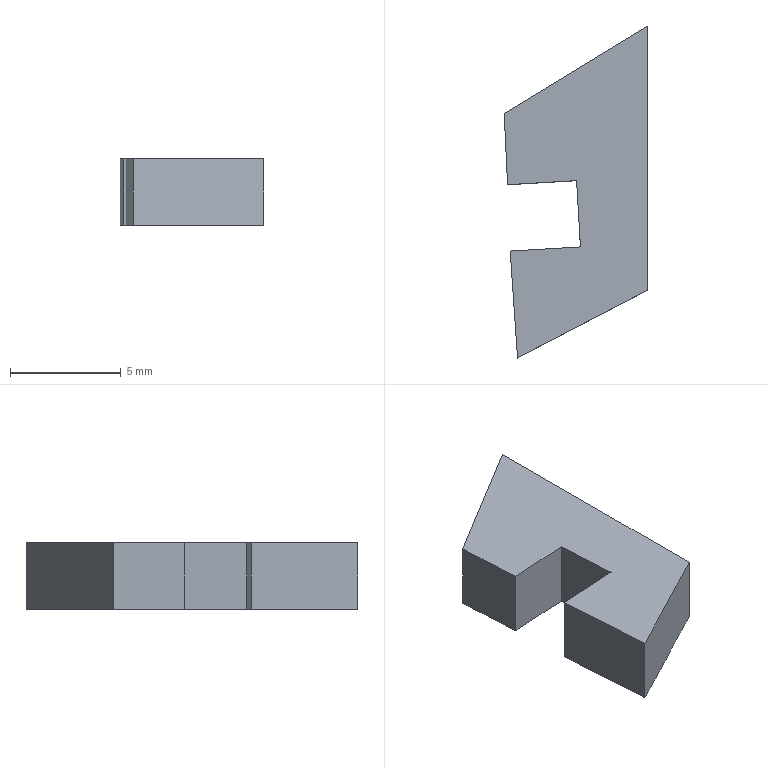Part | SolidWorks | features BaseBody 1 | 1 solid | 10 faces | box 6.477 x 14.965 x 3 mm | volume 188.364 mm3 | plane 10
STEP:
#1=CARTESIAN_POINT('',(10.676,5.598,-1.5));
#2=VERTEX_POINT('',#1);
#3=CARTESIAN_POINT('',(7.509,5.413,-1.5));
#4=VERTEX_POINT('',#3);
#5=CARTESIAN_POINT('',(7.509,5.413,-1.5));
#6=DIRECTION('',(-0.9983,-0.05835,0.));
#7=VECTOR('',#6,1000.);
#8=LINE('',#5,#7);
#9=EDGE_CURVE('',#2,#4,#8,.T.);
#10=ORIENTED_EDGE('',*,*,#9,.F.);
#11=CARTESIAN_POINT('',(10.501,8.588,-1.5));
#12=VERTEX_POINT('',#11);
#13=CARTESIAN_POINT('',(10.676,5.598,-1.5));
#14=DIRECTION('',(0.05835,-0.9983,0.));
#15=VECTOR('',#14,1000.);
#16=LINE('',#13,#15);
#17=EDGE_CURVE('',#12,#2,#16,.T.);
#18=ORIENTED_EDGE('',*,*,#17,.F.);
#19=CARTESIAN_POINT('',(7.389,8.407,-1.5));
#20=VERTEX_POINT('',#19);
#21=CARTESIAN_POINT('',(10.501,8.588,-1.5));
#22=DIRECTION('',(0.9983,0.05835,0.));
#23=VECTOR('',#22,1000.);
#24=LINE('',#21,#23);
#25=EDGE_CURVE('',#20,#12,#24,.T.);
#26=ORIENTED_EDGE('',*,*,#25,.F.);
#27=CARTESIAN_POINT('',(7.239,11.616,-1.5));
#28=VERTEX_POINT('',#27);
#29=CARTESIAN_POINT('',(7.389,8.407,-1.5));
#30=DIRECTION('',(0.04694,-0.9989,0.));
#31=VECTOR('',#30,1000.);
#32=LINE('',#29,#31);
#33=EDGE_CURVE('',#28,#20,#32,.T.);
#34=ORIENTED_EDGE('',*,*,#33,.F.);
#35=CARTESIAN_POINT('',(13.715,15.561,-1.5));
#36=VERTEX_POINT('',#35);
#37=CARTESIAN_POINT('',(7.239,11.616,-1.5));
#38=DIRECTION('',(-0.854,-0.5202,0.));
#39=VECTOR('',#38,1000.);
#40=LINE('',#37,#39);
#41=EDGE_CURVE('',#36,#28,#40,.T.);
#42=ORIENTED_EDGE('',*,*,#41,.F.);
#43=CARTESIAN_POINT('',(13.715,3.649,-1.5));
#44=VERTEX_POINT('',#43);
#45=CARTESIAN_POINT('',(13.715,15.561,-1.5));
#46=DIRECTION('',(0.,1.,0.));
#47=VECTOR('',#46,1000.);
#48=LINE('',#45,#47);
#49=EDGE_CURVE('',#44,#36,#48,.T.);
#50=ORIENTED_EDGE('',*,*,#49,.F.);
#51=CARTESIAN_POINT('',(7.839,0.5953,-1.5));
#52=VERTEX_POINT('',#51);
#53=CARTESIAN_POINT('',(13.715,3.649,-1.5));
#54=DIRECTION('',(0.8874,0.4611,0.));
#55=VECTOR('',#54,1000.);
#56=LINE('',#53,#55);
#57=EDGE_CURVE('',#52,#44,#56,.T.);
#58=ORIENTED_EDGE('',*,*,#57,.F.);
#59=CARTESIAN_POINT('',(7.839,0.5953,-1.5));
#60=DIRECTION('',(0.06826,-0.9977,0.));
#61=VECTOR('',#60,1000.);
#62=LINE('',#59,#61);
#63=EDGE_CURVE('',#4,#52,#62,.T.);
#64=ORIENTED_EDGE('',*,*,#63,.F.);
#65=EDGE_LOOP('',(#10,#18,#26,#34,#42,#50,#58,#64));
#66=FACE_OUTER_BOUND('',#65,.T.);
#67=CARTESIAN_POINT('',(0.,0.,-1.5));
#68=DIRECTION('',(0.,0.,1.));
#69=DIRECTION('',(1.,0.,0.));
#70=AXIS2_PLACEMENT_3D('',#67,#68,#69);
#71=PLANE('',#70);
#72=ADVANCED_FACE('',(#66),#71,.F.);
#73=CARTESIAN_POINT('',(10.676,5.598,1.5));
#74=VERTEX_POINT('',#73);
#75=CARTESIAN_POINT('',(7.509,5.413,1.5));
#76=VERTEX_POINT('',#75);
#77=CARTESIAN_POINT('',(7.509,5.413,1.5));
#78=DIRECTION('',(-0.9983,-0.05835,0.));
#79=VECTOR('',#78,1000.);
#80=LINE('',#77,#79);
#81=EDGE_CURVE('',#74,#76,#80,.T.);
#82=ORIENTED_EDGE('',*,*,#81,.T.);
#83=CARTESIAN_POINT('',(7.839,0.5953,1.5));
#84=VERTEX_POINT('',#83);
#85=CARTESIAN_POINT('',(7.839,0.5953,1.5));
#86=DIRECTION('',(0.06826,-0.9977,0.));
#87=VECTOR('',#86,1000.);
#88=LINE('',#85,#87);
#89=EDGE_CURVE('',#76,#84,#88,.T.);
#90=ORIENTED_EDGE('',*,*,#89,.T.);
#91=CARTESIAN_POINT('',(13.715,3.649,1.5));
#92=VERTEX_POINT('',#91);
#93=CARTESIAN_POINT('',(13.715,3.649,1.5));
#94=DIRECTION('',(0.8874,0.4611,0.));
#95=VECTOR('',#94,1000.);
#96=LINE('',#93,#95);
#97=EDGE_CURVE('',#84,#92,#96,.T.);
#98=ORIENTED_EDGE('',*,*,#97,.T.);
#99=CARTESIAN_POINT('',(13.715,15.561,1.5));
#100=VERTEX_POINT('',#99);
#101=CARTESIAN_POINT('',(13.715,15.561,1.5));
#102=DIRECTION('',(0.,1.,0.));
#103=VECTOR('',#102,1000.);
#104=LINE('',#101,#103);
#105=EDGE_CURVE('',#92,#100,#104,.T.);
#106=ORIENTED_EDGE('',*,*,#105,.T.);
#107=CARTESIAN_POINT('',(7.239,11.616,1.5));
#108=VERTEX_POINT('',#107);
#109=CARTESIAN_POINT('',(7.239,11.616,1.5));
#110=DIRECTION('',(-0.854,-0.5202,0.));
#111=VECTOR('',#110,1000.);
#112=LINE('',#109,#111);
#113=EDGE_CURVE('',#100,#108,#112,.T.);
#114=ORIENTED_EDGE('',*,*,#113,.T.);
#115=CARTESIAN_POINT('',(7.389,8.407,1.5));
#116=VERTEX_POINT('',#115);
#117=CARTESIAN_POINT('',(7.389,8.407,1.5));
#118=DIRECTION('',(0.04694,-0.9989,0.));
#119=VECTOR('',#118,1000.);
#120=LINE('',#117,#119);
#121=EDGE_CURVE('',#108,#116,#120,.T.);
#122=ORIENTED_EDGE('',*,*,#121,.T.);
#123=CARTESIAN_POINT('',(10.501,8.588,1.5));
#124=VERTEX_POINT('',#123);
#125=CARTESIAN_POINT('',(10.501,8.588,1.5));
#126=DIRECTION('',(0.9983,0.05835,0.));
#127=VECTOR('',#126,1000.);
#128=LINE('',#125,#127);
#129=EDGE_CURVE('',#116,#124,#128,.T.);
#130=ORIENTED_EDGE('',*,*,#129,.T.);
#131=CARTESIAN_POINT('',(10.676,5.598,1.5));
#132=DIRECTION('',(0.05835,-0.9983,0.));
#133=VECTOR('',#132,1000.);
#134=LINE('',#131,#133);
#135=EDGE_CURVE('',#124,#74,#134,.T.);
#136=ORIENTED_EDGE('',*,*,#135,.T.);
#137=EDGE_LOOP('',(#82,#90,#98,#106,#114,#122,#130,#136));
#138=FACE_OUTER_BOUND('',#137,.T.);
#139=CARTESIAN_POINT('',(0.,0.,1.5));
#140=DIRECTION('',(0.,0.,1.));
#141=DIRECTION('',(1.,0.,0.));
#142=AXIS2_PLACEMENT_3D('',#139,#140,#141);
#143=PLANE('',#142);
#144=ADVANCED_FACE('',(#138),#143,.T.);
#145=ORIENTED_EDGE('',*,*,#17,.T.);
#146=CARTESIAN_POINT('',(10.676,5.598,1.5));
#147=DIRECTION('',(0.,0.,-1.));
#148=VECTOR('',#147,1000.);
#149=LINE('',#146,#148);
#150=EDGE_CURVE('',#74,#2,#149,.T.);
#151=ORIENTED_EDGE('',*,*,#150,.F.);
#152=ORIENTED_EDGE('',*,*,#135,.F.);
#153=CARTESIAN_POINT('',(10.501,8.588,1.5));
#154=DIRECTION('',(0.,0.,-1.));
#155=VECTOR('',#154,1000.);
#156=LINE('',#153,#155);
#157=EDGE_CURVE('',#124,#12,#156,.T.);
#158=ORIENTED_EDGE('',*,*,#157,.T.);
#159=EDGE_LOOP('',(#145,#151,#152,#158));
#160=FACE_OUTER_BOUND('',#159,.T.);
#161=CARTESIAN_POINT('',(10.676,5.598,1.5));
#162=DIRECTION('',(0.9983,0.05835,0.));
#163=DIRECTION('',(0.,0.,-1.));
#164=AXIS2_PLACEMENT_3D('',#161,#162,#163);
#165=PLANE('',#164);
#166=ADVANCED_FACE('',(#160),#165,.F.);
#167=ORIENTED_EDGE('',*,*,#25,.T.);
#168=ORIENTED_EDGE('',*,*,#157,.F.);
#169=ORIENTED_EDGE('',*,*,#129,.F.);
#170=CARTESIAN_POINT('',(7.389,8.407,1.5));
#171=DIRECTION('',(0.,0.,-1.));
#172=VECTOR('',#171,1000.);
#173=LINE('',#170,#172);
#174=EDGE_CURVE('',#116,#20,#173,.T.);
#175=ORIENTED_EDGE('',*,*,#174,.T.);
#176=EDGE_LOOP('',(#167,#168,#169,#175));
#177=FACE_OUTER_BOUND('',#176,.T.);
#178=CARTESIAN_POINT('',(10.501,8.588,1.5));
#179=DIRECTION('',(-0.05835,0.9983,0.));
#180=DIRECTION('',(0.,0.,1.));
#181=AXIS2_PLACEMENT_3D('',#178,#179,#180);
#182=PLANE('',#181);
#183=ADVANCED_FACE('',(#177),#182,.F.);
#184=ORIENTED_EDGE('',*,*,#33,.T.);
#185=ORIENTED_EDGE('',*,*,#174,.F.);
#186=ORIENTED_EDGE('',*,*,#121,.F.);
#187=CARTESIAN_POINT('',(7.239,11.616,1.5));
#188=DIRECTION('',(0.,0.,-1.));
#189=VECTOR('',#188,1000.);
#190=LINE('',#187,#189);
#191=EDGE_CURVE('',#108,#28,#190,.T.);
#192=ORIENTED_EDGE('',*,*,#191,.T.);
#193=EDGE_LOOP('',(#184,#185,#186,#192));
#194=FACE_OUTER_BOUND('',#193,.T.);
#195=CARTESIAN_POINT('',(7.389,8.407,1.5));
#196=DIRECTION('',(0.9989,0.04694,0.));
#197=DIRECTION('',(0.,0.,-1.));
#198=AXIS2_PLACEMENT_3D('',#195,#196,#197);
#199=PLANE('',#198);
#200=ADVANCED_FACE('',(#194),#199,.F.);
#201=ORIENTED_EDGE('',*,*,#41,.T.);
#202=ORIENTED_EDGE('',*,*,#191,.F.);
#203=ORIENTED_EDGE('',*,*,#113,.F.);
#204=CARTESIAN_POINT('',(13.715,15.561,1.5));
#205=DIRECTION('',(0.,0.,-1.));
#206=VECTOR('',#205,1000.);
#207=LINE('',#204,#206);
#208=EDGE_CURVE('',#100,#36,#207,.T.);
#209=ORIENTED_EDGE('',*,*,#208,.T.);
#210=EDGE_LOOP('',(#201,#202,#203,#209));
#211=FACE_OUTER_BOUND('',#210,.T.);
#212=CARTESIAN_POINT('',(7.239,11.616,1.5));
#213=DIRECTION('',(0.5202,-0.854,0.));
#214=DIRECTION('',(0.,0.,-1.));
#215=AXIS2_PLACEMENT_3D('',#212,#213,#214);
#216=PLANE('',#215);
#217=ADVANCED_FACE('',(#211),#216,.F.);
#218=ORIENTED_EDGE('',*,*,#49,.T.);
#219=ORIENTED_EDGE('',*,*,#208,.F.);
#220=ORIENTED_EDGE('',*,*,#105,.F.);
#221=CARTESIAN_POINT('',(13.715,3.649,1.5));
#222=DIRECTION('',(0.,0.,-1.));
#223=VECTOR('',#222,1000.);
#224=LINE('',#221,#223);
#225=EDGE_CURVE('',#92,#44,#224,.T.);
#226=ORIENTED_EDGE('',*,*,#225,.T.);
#227=EDGE_LOOP('',(#218,#219,#220,#226));
#228=FACE_OUTER_BOUND('',#227,.T.);
#229=CARTESIAN_POINT('',(13.715,15.561,1.5));
#230=DIRECTION('',(-1.,0.,0.));
#231=DIRECTION('',(0.,0.,1.));
#232=AXIS2_PLACEMENT_3D('',#229,#230,#231);
#233=PLANE('',#232);
#234=ADVANCED_FACE('',(#228),#233,.F.);
#235=ORIENTED_EDGE('',*,*,#57,.T.);
#236=ORIENTED_EDGE('',*,*,#225,.F.);
#237=ORIENTED_EDGE('',*,*,#97,.F.);
#238=CARTESIAN_POINT('',(7.839,0.5953,1.5));
#239=DIRECTION('',(0.,0.,-1.));
#240=VECTOR('',#239,1000.);
#241=LINE('',#238,#240);
#242=EDGE_CURVE('',#84,#52,#241,.T.);
#243=ORIENTED_EDGE('',*,*,#242,.T.);
#244=EDGE_LOOP('',(#235,#236,#237,#243));
#245=FACE_OUTER_BOUND('',#244,.T.);
#246=CARTESIAN_POINT('',(13.715,3.649,1.5));
#247=DIRECTION('',(-0.4611,0.8874,0.));
#248=DIRECTION('',(0.,0.,1.));
#249=AXIS2_PLACEMENT_3D('',#246,#247,#248);
#250=PLANE('',#249);
#251=ADVANCED_FACE('',(#245),#250,.F.);
#252=ORIENTED_EDGE('',*,*,#63,.T.);
#253=ORIENTED_EDGE('',*,*,#242,.F.);
#254=ORIENTED_EDGE('',*,*,#89,.F.);
#255=CARTESIAN_POINT('',(7.509,5.413,1.5));
#256=DIRECTION('',(0.,0.,-1.));
#257=VECTOR('',#256,1000.);
#258=LINE('',#255,#257);
#259=EDGE_CURVE('',#76,#4,#258,.T.);
#260=ORIENTED_EDGE('',*,*,#259,.T.);
#261=EDGE_LOOP('',(#252,#253,#254,#260));
#262=FACE_OUTER_BOUND('',#261,.T.);
#263=CARTESIAN_POINT('',(7.839,0.5953,1.5));
#264=DIRECTION('',(0.9977,0.06826,0.));
#265=DIRECTION('',(0.,0.,-1.));
#266=AXIS2_PLACEMENT_3D('',#263,#264,#265);
#267=PLANE('',#266);
#268=ADVANCED_FACE('',(#262),#267,.F.);
#269=ORIENTED_EDGE('',*,*,#9,.T.);
#270=ORIENTED_EDGE('',*,*,#259,.F.);
#271=ORIENTED_EDGE('',*,*,#81,.F.);
#272=ORIENTED_EDGE('',*,*,#150,.T.);
#273=EDGE_LOOP('',(#269,#270,#271,#272));
#274=FACE_OUTER_BOUND('',#273,.T.);
#275=CARTESIAN_POINT('',(7.509,5.413,1.5));
#276=DIRECTION('',(0.05835,-0.9983,0.));
#277=DIRECTION('',(0.,0.,-1.));
#278=AXIS2_PLACEMENT_3D('',#275,#276,#277);
#279=PLANE('',#278);
#280=ADVANCED_FACE('',(#274),#279,.F.);
#281=CLOSED_SHELL('',(#72,#144,#166,#183,#200,#217,#234,#251,#268,#280));
#282=MANIFOLD_SOLID_BREP('',#281);
#283=CARTESIAN_POINT('',(0.,0.,0.));
#284=DIRECTION('',(0.,0.,1.));
#285=DIRECTION('',(1.,0.,0.));
#286=AXIS2_PLACEMENT_3D('',#283,#284,#285);
#287=(LENGTH_UNIT()NAMED_UNIT(*)SI_UNIT(.MILLI.,.METRE.));
#288=UNCERTAINTY_MEASURE_WITH_UNIT(LENGTH_MEASURE(0.00001),#287,'','');
#289=(NAMED_UNIT(*)PLANE_ANGLE_UNIT()SI_UNIT($,.RADIAN.));
#290=(NAMED_UNIT(*)SI_UNIT($,.STERADIAN.)SOLID_ANGLE_UNIT());
#291=(GEOMETRIC_REPRESENTATION_CONTEXT(3)GLOBAL_UNCERTAINTY_ASSIGNED_CONTEXT((#288))GLOBAL_UNIT_ASSIGNED_CONTEXT((#287,#289,#290))REPRESENTATION_CONTEXT('',''));
#292=ADVANCED_BREP_SHAPE_REPRESENTATION('',(#282,#286),#291);